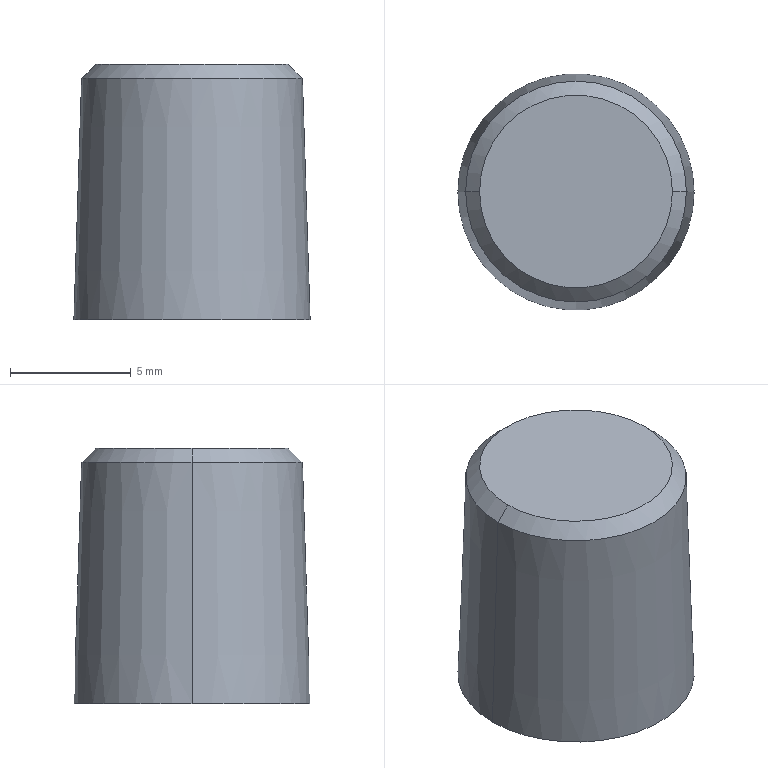Part | Creo | 1 solid | 13 faces | box 9.8 x 9.8 x 10.58 mm | volume 677.314 mm3 | plane 9 | cone 4
STEP:
#1=CARTESIAN_POINT('',(0.,0.,0.));
#2=DIRECTION('',(0.,0.,1.));
#3=DIRECTION('',(1.,0.,0.));
#4=AXIS2_PLACEMENT_3D('',#1,#2,#3);
#5=CARTESIAN_POINT('',(-64.9,75.6,-7.827));
#6=VERTEX_POINT('',#5);
#7=CARTESIAN_POINT('',(-55.1,75.6,-7.827));
#8=VERTEX_POINT('',#7);
#9=CARTESIAN_POINT('',(-60.,75.6,-7.827));
#10=DIRECTION('',(0.,0.,-1.));
#11=DIRECTION('',(-1.,0.,0.));
#12=AXIS2_PLACEMENT_3D('',#9,#10,#11);
#13=CIRCLE('',#12,4.9);
#14=EDGE_CURVE('',#6,#8,#13,.T.);
#15=ORIENTED_EDGE('',*,*,#14,.F.);
#16=CARTESIAN_POINT('',(-60.,75.6,-7.827));
#17=DIRECTION('',(0.,0.,-1.));
#18=DIRECTION('',(1.,0.,0.));
#19=AXIS2_PLACEMENT_3D('',#16,#17,#18);
#20=CIRCLE('',#19,4.9);
#21=EDGE_CURVE('',#8,#6,#20,.T.);
#22=ORIENTED_EDGE('',*,*,#21,.F.);
#23=EDGE_LOOP('',(#15,#22));
#24=FACE_OUTER_BOUND('',#23,.F.);
#25=CARTESIAN_POINT('',(-57.55,77.015,-7.827));
#26=VERTEX_POINT('',#25);
#27=CARTESIAN_POINT('',(-60.,78.429,-7.827));
#28=VERTEX_POINT('',#27);
#29=CARTESIAN_POINT('',(-57.55,77.015,-7.827));
#30=DIRECTION('',(-0.866,0.5,0.));
#31=VECTOR('',#30,2.829);
#32=LINE('',#29,#31);
#33=EDGE_CURVE('',#26,#28,#32,.T.);
#34=ORIENTED_EDGE('',*,*,#33,.F.);
#35=CARTESIAN_POINT('',(-57.55,74.185,-7.827));
#36=VERTEX_POINT('',#35);
#37=CARTESIAN_POINT('',(-57.55,77.015,-7.827));
#38=DIRECTION('',(0.,-1.,0.));
#39=VECTOR('',#38,2.829);
#40=LINE('',#37,#39);
#41=EDGE_CURVE('',#26,#36,#40,.T.);
#42=ORIENTED_EDGE('',*,*,#41,.T.);
#43=CARTESIAN_POINT('',(-60.,72.771,-7.827));
#44=VERTEX_POINT('',#43);
#45=CARTESIAN_POINT('',(-60.,72.771,-7.827));
#46=DIRECTION('',(0.866,0.5,0.));
#47=VECTOR('',#46,2.829);
#48=LINE('',#45,#47);
#49=EDGE_CURVE('',#44,#36,#48,.T.);
#50=ORIENTED_EDGE('',*,*,#49,.F.);
#51=CARTESIAN_POINT('',(-62.45,74.185,-7.827));
#52=VERTEX_POINT('',#51);
#53=CARTESIAN_POINT('',(-62.45,74.185,-7.827));
#54=DIRECTION('',(0.866,-0.5,0.));
#55=VECTOR('',#54,2.829);
#56=LINE('',#53,#55);
#57=EDGE_CURVE('',#52,#44,#56,.T.);
#58=ORIENTED_EDGE('',*,*,#57,.F.);
#59=CARTESIAN_POINT('',(-62.45,77.015,-7.827));
#60=VERTEX_POINT('',#59);
#61=CARTESIAN_POINT('',(-62.45,74.185,-7.827));
#62=DIRECTION('',(0.,1.,0.));
#63=VECTOR('',#62,2.829);
#64=LINE('',#61,#63);
#65=EDGE_CURVE('',#52,#60,#64,.T.);
#66=ORIENTED_EDGE('',*,*,#65,.T.);
#67=CARTESIAN_POINT('',(-60.,78.429,-7.827));
#68=DIRECTION('',(-0.866,-0.5,0.));
#69=VECTOR('',#68,2.829);
#70=LINE('',#67,#69);
#71=EDGE_CURVE('',#28,#60,#70,.T.);
#72=ORIENTED_EDGE('',*,*,#71,.F.);
#73=EDGE_LOOP('',(#34,#42,#50,#58,#66,#72));
#74=FACE_BOUND('',#73,.F.);
#75=CARTESIAN_POINT('',(-60.,75.6,-7.827));
#76=DIRECTION('',(0.,0.,-1.));
#77=DIRECTION('',(0.,1.,0.));
#78=AXIS2_PLACEMENT_3D('',#75,#76,#77);
#79=PLANE('',#78);
#80=ADVANCED_FACE('',(#24,#74),#79,.T.);
#81=CARTESIAN_POINT('',(-64.58,75.6,2.172));
#82=VERTEX_POINT('',#81);
#83=CARTESIAN_POINT('',(-55.42,75.6,2.172));
#84=VERTEX_POINT('',#83);
#85=CARTESIAN_POINT('',(-60.,75.6,2.172));
#86=DIRECTION('',(0.,0.,-1.));
#87=DIRECTION('',(-1.,0.,0.));
#88=AXIS2_PLACEMENT_3D('',#85,#86,#87);
#89=CIRCLE('',#88,4.58);
#90=EDGE_CURVE('',#82,#84,#89,.T.);
#91=ORIENTED_EDGE('',*,*,#90,.F.);
#92=CARTESIAN_POINT('',(-64.58,75.6,2.172));
#93=DIRECTION('',(-0.03198,0.,-0.9995));
#94=VECTOR('',#93,10.005);
#95=LINE('',#92,#94);
#96=EDGE_CURVE('',#82,#6,#95,.T.);
#97=ORIENTED_EDGE('',*,*,#96,.T.);
#98=ORIENTED_EDGE('',*,*,#14,.T.);
#99=CARTESIAN_POINT('',(-55.42,75.6,2.172));
#100=DIRECTION('',(0.03198,0.,-0.9995));
#101=VECTOR('',#100,10.005);
#102=LINE('',#99,#101);
#103=EDGE_CURVE('',#84,#8,#102,.T.);
#104=ORIENTED_EDGE('',*,*,#103,.F.);
#105=EDGE_LOOP('',(#91,#97,#98,#104));
#106=FACE_OUTER_BOUND('',#105,.F.);
#107=CARTESIAN_POINT('',(-60.,75.6,-2.828));
#108=DIRECTION('',(0.,0.,-1.));
#109=DIRECTION('',(-1.,0.,0.));
#110=AXIS2_PLACEMENT_3D('',#107,#108,#109);
#111=CONICAL_SURFACE('',#110,4.74,1.833);
#112=ADVANCED_FACE('',(#106),#111,.T.);
#113=CARTESIAN_POINT('',(-56.,75.6,2.752));
#114=VERTEX_POINT('',#113);
#115=CARTESIAN_POINT('',(-64.,75.6,2.752));
#116=VERTEX_POINT('',#115);
#117=CARTESIAN_POINT('',(-60.,75.6,2.752));
#118=DIRECTION('',(0.,0.,1.));
#119=DIRECTION('',(1.,0.,0.));
#120=AXIS2_PLACEMENT_3D('',#117,#118,#119);
#121=CIRCLE('',#120,4.);
#122=EDGE_CURVE('',#114,#116,#121,.T.);
#123=ORIENTED_EDGE('',*,*,#122,.T.);
#124=CARTESIAN_POINT('',(-64.,75.6,2.752));
#125=DIRECTION('',(-0.7071,0.,-0.7071));
#126=VECTOR('',#125,0.8202);
#127=LINE('',#124,#126);
#128=EDGE_CURVE('',#116,#82,#127,.T.);
#129=ORIENTED_EDGE('',*,*,#128,.T.);
#130=ORIENTED_EDGE('',*,*,#90,.T.);
#131=CARTESIAN_POINT('',(-56.,75.6,2.752));
#132=DIRECTION('',(0.7071,0.,-0.7071));
#133=VECTOR('',#132,0.8202);
#134=LINE('',#131,#133);
#135=EDGE_CURVE('',#114,#84,#134,.T.);
#136=ORIENTED_EDGE('',*,*,#135,.F.);
#137=EDGE_LOOP('',(#123,#129,#130,#136));
#138=FACE_OUTER_BOUND('',#137,.F.);
#139=CARTESIAN_POINT('',(-60.,75.6,2.462));
#140=DIRECTION('',(0.,0.,-1.));
#141=DIRECTION('',(-1.,0.,0.));
#142=AXIS2_PLACEMENT_3D('',#139,#140,#141);
#143=CONICAL_SURFACE('',#142,4.29,45.);
#144=ADVANCED_FACE('',(#138),#143,.T.);
#145=CARTESIAN_POINT('',(-60.,75.6,2.752));
#146=DIRECTION('',(0.,0.,1.));
#147=DIRECTION('',(-1.,0.,0.));
#148=AXIS2_PLACEMENT_3D('',#145,#146,#147);
#149=CIRCLE('',#148,4.);
#150=EDGE_CURVE('',#116,#114,#149,.T.);
#151=ORIENTED_EDGE('',*,*,#150,.F.);
#152=ORIENTED_EDGE('',*,*,#122,.F.);
#153=EDGE_LOOP('',(#151,#152));
#154=FACE_OUTER_BOUND('',#153,.F.);
#155=CARTESIAN_POINT('',(-60.,75.6,2.752));
#156=DIRECTION('',(0.,0.,1.));
#157=DIRECTION('',(0.,-1.,0.));
#158=AXIS2_PLACEMENT_3D('',#155,#156,#157);
#159=PLANE('',#158);
#160=ADVANCED_FACE('',(#154),#159,.T.);
#161=ORIENTED_EDGE('',*,*,#150,.T.);
#162=ORIENTED_EDGE('',*,*,#135,.T.);
#163=CARTESIAN_POINT('',(-60.,75.6,2.172));
#164=DIRECTION('',(0.,0.,-1.));
#165=DIRECTION('',(1.,0.,0.));
#166=AXIS2_PLACEMENT_3D('',#163,#164,#165);
#167=CIRCLE('',#166,4.58);
#168=EDGE_CURVE('',#84,#82,#167,.T.);
#169=ORIENTED_EDGE('',*,*,#168,.T.);
#170=ORIENTED_EDGE('',*,*,#128,.F.);
#171=EDGE_LOOP('',(#161,#162,#169,#170));
#172=FACE_OUTER_BOUND('',#171,.F.);
#173=CARTESIAN_POINT('',(-60.,75.6,2.462));
#174=DIRECTION('',(0.,0.,-1.));
#175=DIRECTION('',(-1.,0.,0.));
#176=AXIS2_PLACEMENT_3D('',#173,#174,#175);
#177=CONICAL_SURFACE('',#176,4.29,45.);
#178=ADVANCED_FACE('',(#172),#177,.T.);
#179=ORIENTED_EDGE('',*,*,#168,.F.);
#180=ORIENTED_EDGE('',*,*,#103,.T.);
#181=ORIENTED_EDGE('',*,*,#21,.T.);
#182=ORIENTED_EDGE('',*,*,#96,.F.);
#183=EDGE_LOOP('',(#179,#180,#181,#182));
#184=FACE_OUTER_BOUND('',#183,.F.);
#185=CARTESIAN_POINT('',(-60.,75.6,-2.828));
#186=DIRECTION('',(0.,0.,-1.));
#187=DIRECTION('',(-1.,0.,0.));
#188=AXIS2_PLACEMENT_3D('',#185,#186,#187);
#189=CONICAL_SURFACE('',#188,4.74,1.833);
#190=ADVANCED_FACE('',(#184),#189,.T.);
#191=CARTESIAN_POINT('',(-60.,78.429,-4.827));
#192=VERTEX_POINT('',#191);
#193=CARTESIAN_POINT('',(-57.55,77.015,-4.827));
#194=VERTEX_POINT('',#193);
#195=CARTESIAN_POINT('',(-60.,78.429,-4.827));
#196=DIRECTION('',(0.866,-0.5,0.));
#197=VECTOR('',#196,2.829);
#198=LINE('',#195,#197);
#199=EDGE_CURVE('',#192,#194,#198,.T.);
#200=ORIENTED_EDGE('',*,*,#199,.T.);
#201=CARTESIAN_POINT('',(-57.55,77.015,-7.827));
#202=DIRECTION('',(0.,0.,1.));
#203=VECTOR('',#202,3.);
#204=LINE('',#201,#203);
#205=EDGE_CURVE('',#26,#194,#204,.T.);
#206=ORIENTED_EDGE('',*,*,#205,.F.);
#207=ORIENTED_EDGE('',*,*,#33,.T.);
#208=CARTESIAN_POINT('',(-60.,78.429,-7.827));
#209=DIRECTION('',(0.,0.,1.));
#210=VECTOR('',#209,3.);
#211=LINE('',#208,#210);
#212=EDGE_CURVE('',#28,#192,#211,.T.);
#213=ORIENTED_EDGE('',*,*,#212,.T.);
#214=EDGE_LOOP('',(#200,#206,#207,#213));
#215=FACE_OUTER_BOUND('',#214,.F.);
#216=CARTESIAN_POINT('',(-58.775,77.722,-6.327));
#217=DIRECTION('',(0.5,0.866,0.));
#218=DIRECTION('',(-0.866,0.5,0.));
#219=AXIS2_PLACEMENT_3D('',#216,#217,#218);
#220=PLANE('',#219);
#221=ADVANCED_FACE('',(#215),#220,.F.);
#222=CARTESIAN_POINT('',(-57.55,74.185,-4.827));
#223=VERTEX_POINT('',#222);
#224=CARTESIAN_POINT('',(-57.55,74.185,-4.827));
#225=DIRECTION('',(0.,1.,0.));
#226=VECTOR('',#225,2.829);
#227=LINE('',#224,#226);
#228=EDGE_CURVE('',#223,#194,#227,.T.);
#229=ORIENTED_EDGE('',*,*,#228,.T.);
#230=ORIENTED_EDGE('',*,*,#199,.F.);
#231=CARTESIAN_POINT('',(-62.45,77.015,-4.827));
#232=VERTEX_POINT('',#231);
#233=CARTESIAN_POINT('',(-62.45,77.015,-4.827));
#234=DIRECTION('',(0.866,0.5,0.));
#235=VECTOR('',#234,2.829);
#236=LINE('',#233,#235);
#237=EDGE_CURVE('',#232,#192,#236,.T.);
#238=ORIENTED_EDGE('',*,*,#237,.F.);
#239=CARTESIAN_POINT('',(-62.45,74.185,-4.827));
#240=VERTEX_POINT('',#239);
#241=CARTESIAN_POINT('',(-62.45,77.015,-4.827));
#242=DIRECTION('',(0.,-1.,0.));
#243=VECTOR('',#242,2.829);
#244=LINE('',#241,#243);
#245=EDGE_CURVE('',#232,#240,#244,.T.);
#246=ORIENTED_EDGE('',*,*,#245,.T.);
#247=CARTESIAN_POINT('',(-60.,72.771,-4.827));
#248=VERTEX_POINT('',#247);
#249=CARTESIAN_POINT('',(-60.,72.771,-4.827));
#250=DIRECTION('',(-0.866,0.5,0.));
#251=VECTOR('',#250,2.829);
#252=LINE('',#249,#251);
#253=EDGE_CURVE('',#248,#240,#252,.T.);
#254=ORIENTED_EDGE('',*,*,#253,.F.);
#255=CARTESIAN_POINT('',(-57.55,74.185,-4.827));
#256=DIRECTION('',(-0.866,-0.5,0.));
#257=VECTOR('',#256,2.829);
#258=LINE('',#255,#257);
#259=EDGE_CURVE('',#223,#248,#258,.T.);
#260=ORIENTED_EDGE('',*,*,#259,.F.);
#261=EDGE_LOOP('',(#229,#230,#238,#246,#254,#260));
#262=FACE_OUTER_BOUND('',#261,.F.);
#263=CARTESIAN_POINT('',(-60.,75.6,-4.827));
#264=DIRECTION('',(0.,0.,1.));
#265=DIRECTION('',(0.,1.,0.));
#266=AXIS2_PLACEMENT_3D('',#263,#264,#265);
#267=PLANE('',#266);
#268=ADVANCED_FACE('',(#262),#267,.F.);
#269=ORIENTED_EDGE('',*,*,#228,.F.);
#270=CARTESIAN_POINT('',(-57.55,74.185,-7.827));
#271=DIRECTION('',(0.,0.,1.));
#272=VECTOR('',#271,3.);
#273=LINE('',#270,#272);
#274=EDGE_CURVE('',#36,#223,#273,.T.);
#275=ORIENTED_EDGE('',*,*,#274,.F.);
#276=ORIENTED_EDGE('',*,*,#41,.F.);
#277=ORIENTED_EDGE('',*,*,#205,.T.);
#278=EDGE_LOOP('',(#269,#275,#276,#277));
#279=FACE_OUTER_BOUND('',#278,.F.);
#280=CARTESIAN_POINT('',(-57.55,75.6,-6.327));
#281=DIRECTION('',(1.,0.,0.));
#282=DIRECTION('',(0.,0.,1.));
#283=AXIS2_PLACEMENT_3D('',#280,#281,#282);
#284=PLANE('',#283);
#285=ADVANCED_FACE('',(#279),#284,.F.);
#286=ORIENTED_EDGE('',*,*,#259,.T.);
#287=CARTESIAN_POINT('',(-60.,72.771,-7.827));
#288=DIRECTION('',(0.,0.,1.));
#289=VECTOR('',#288,3.);
#290=LINE('',#287,#289);
#291=EDGE_CURVE('',#44,#248,#290,.T.);
#292=ORIENTED_EDGE('',*,*,#291,.F.);
#293=ORIENTED_EDGE('',*,*,#49,.T.);
#294=ORIENTED_EDGE('',*,*,#274,.T.);
#295=EDGE_LOOP('',(#286,#292,#293,#294));
#296=FACE_OUTER_BOUND('',#295,.F.);
#297=CARTESIAN_POINT('',(-58.775,73.478,-6.327));
#298=DIRECTION('',(0.5,-0.866,0.));
#299=DIRECTION('',(0.866,0.5,0.));
#300=AXIS2_PLACEMENT_3D('',#297,#298,#299);
#301=PLANE('',#300);
#302=ADVANCED_FACE('',(#296),#301,.F.);
#303=ORIENTED_EDGE('',*,*,#253,.T.);
#304=CARTESIAN_POINT('',(-62.45,74.185,-7.827));
#305=DIRECTION('',(0.,0.,1.));
#306=VECTOR('',#305,3.);
#307=LINE('',#304,#306);
#308=EDGE_CURVE('',#52,#240,#307,.T.);
#309=ORIENTED_EDGE('',*,*,#308,.F.);
#310=ORIENTED_EDGE('',*,*,#57,.T.);
#311=ORIENTED_EDGE('',*,*,#291,.T.);
#312=EDGE_LOOP('',(#303,#309,#310,#311));
#313=FACE_OUTER_BOUND('',#312,.F.);
#314=CARTESIAN_POINT('',(-61.225,73.478,-6.327));
#315=DIRECTION('',(-0.5,-0.866,0.));
#316=DIRECTION('',(0.866,-0.5,0.));
#317=AXIS2_PLACEMENT_3D('',#314,#315,#316);
#318=PLANE('',#317);
#319=ADVANCED_FACE('',(#313),#318,.F.);
#320=ORIENTED_EDGE('',*,*,#245,.F.);
#321=CARTESIAN_POINT('',(-62.45,77.015,-7.827));
#322=DIRECTION('',(0.,0.,1.));
#323=VECTOR('',#322,3.);
#324=LINE('',#321,#323);
#325=EDGE_CURVE('',#60,#232,#324,.T.);
#326=ORIENTED_EDGE('',*,*,#325,.F.);
#327=ORIENTED_EDGE('',*,*,#65,.F.);
#328=ORIENTED_EDGE('',*,*,#308,.T.);
#329=EDGE_LOOP('',(#320,#326,#327,#328));
#330=FACE_OUTER_BOUND('',#329,.F.);
#331=CARTESIAN_POINT('',(-62.45,75.6,-6.327));
#332=DIRECTION('',(-1.,0.,0.));
#333=DIRECTION('',(0.,0.,-1.));
#334=AXIS2_PLACEMENT_3D('',#331,#332,#333);
#335=PLANE('',#334);
#336=ADVANCED_FACE('',(#330),#335,.F.);
#337=ORIENTED_EDGE('',*,*,#237,.T.);
#338=ORIENTED_EDGE('',*,*,#212,.F.);
#339=ORIENTED_EDGE('',*,*,#71,.T.);
#340=ORIENTED_EDGE('',*,*,#325,.T.);
#341=EDGE_LOOP('',(#337,#338,#339,#340));
#342=FACE_OUTER_BOUND('',#341,.F.);
#343=CARTESIAN_POINT('',(-61.225,77.722,-6.327));
#344=DIRECTION('',(-0.5,0.866,0.));
#345=DIRECTION('',(-0.866,-0.5,0.));
#346=AXIS2_PLACEMENT_3D('',#343,#344,#345);
#347=PLANE('',#346);
#348=ADVANCED_FACE('',(#342),#347,.F.);
#349=CLOSED_SHELL('',(#80,#112,#144,#160,#178,#190,#221,#268,#285,#302,#319,#336,#348));
#350=MANIFOLD_SOLID_BREP('',#349);
#351=(LENGTH_UNIT()NAMED_UNIT(*)SI_UNIT(.MILLI.,.METRE.));
#352=UNCERTAINTY_MEASURE_WITH_UNIT(LENGTH_MEASURE(0.001744),#351,'','');
#353=(NAMED_UNIT(*)PLANE_ANGLE_UNIT()SI_UNIT($,.RADIAN.));
#354=PLANE_ANGLE_MEASURE_WITH_UNIT(PLANE_ANGLE_MEASURE(0.01745),#353);
#355=(CONVERSION_BASED_UNIT('DEGREE',#354)NAMED_UNIT(*)PLANE_ANGLE_UNIT());
#356=(NAMED_UNIT(*)SI_UNIT($,.STERADIAN.)SOLID_ANGLE_UNIT());
#357=(GEOMETRIC_REPRESENTATION_CONTEXT(3)GLOBAL_UNCERTAINTY_ASSIGNED_CONTEXT((#352))GLOBAL_UNIT_ASSIGNED_CONTEXT((#351,#355,#356))REPRESENTATION_CONTEXT('',''));
#358=ADVANCED_BREP_SHAPE_REPRESENTATION('',(#4,#350),#357);